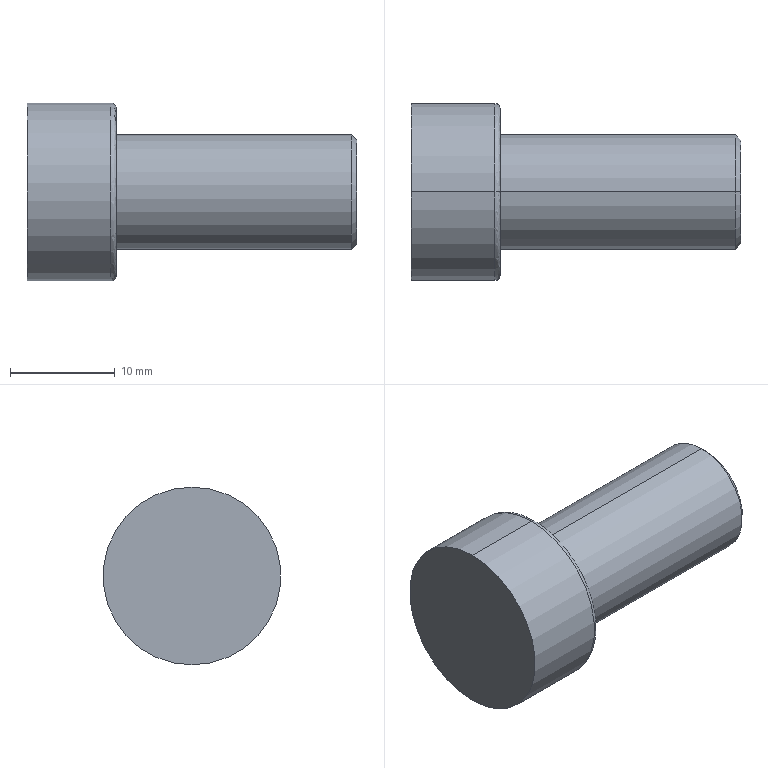Part | STEP file | _BMH070 Welle20 | 1 solid | 22 faces | box 31.5 x 17 x 17 mm | volume 3904 mm3 | cylinder 8 | cone 8 | plane 4 | spline 2 | commonest cylinder face diameters 3.242 x2 5.3 x2 11 x2 17 x2
STEP:
#1=CARTESIAN_POINT('',(8.5,0.,-8.));
#2=VERTEX_POINT('',#1);
#3=CARTESIAN_POINT('',(8.5,0.,8.));
#4=VERTEX_POINT('',#3);
#5=CARTESIAN_POINT('',(8.5,0.,-8.));
#6=CARTESIAN_POINT('',(8.5,-16.,-8.));
#7=CARTESIAN_POINT('',(8.5,-16.,8.));
#8=CARTESIAN_POINT('',(8.5,0.,8.));
#9=(BOUNDED_CURVE()B_SPLINE_CURVE(3,(#5,#6,#7,#8),.UNSPECIFIED.,.F.,.F.)B_SPLINE_CURVE_WITH_KNOTS((4,4),(0.,0.5),.UNSPECIFIED.)CURVE()GEOMETRIC_REPRESENTATION_ITEM()RATIONAL_B_SPLINE_CURVE((1.,0.3333,0.3333,1.))REPRESENTATION_ITEM(''));
#10=EDGE_CURVE('',#2,#4,#9,.T.);
#11=ORIENTED_EDGE('',*,*,#10,.T.);
#12=CARTESIAN_POINT('',(8.,0.,8.5));
#13=VERTEX_POINT('',#12);
#14=CARTESIAN_POINT('',(8.,0.,8.));
#15=DIRECTION('',(0.,-1.,0.));
#16=DIRECTION('',(0.,0.,1.));
#17=AXIS2_PLACEMENT_3D('',#14,#15,#16);
#18=CIRCLE('',#17,0.5);
#19=EDGE_CURVE('',#4,#13,#18,.T.);
#20=ORIENTED_EDGE('',*,*,#19,.T.);
#21=CARTESIAN_POINT('',(8.,0.,-8.5));
#22=VERTEX_POINT('',#21);
#23=CARTESIAN_POINT('',(8.,0.,0.));
#24=DIRECTION('',(1.,0.,0.));
#25=DIRECTION('',(0.,0.,-1.));
#26=AXIS2_PLACEMENT_3D('',#23,#24,#25);
#27=CIRCLE('',#26,8.5);
#28=EDGE_CURVE('',#13,#22,#27,.T.);
#29=ORIENTED_EDGE('',*,*,#28,.T.);
#30=CARTESIAN_POINT('',(8.,0.,-8.));
#31=DIRECTION('',(0.,1.,0.));
#32=DIRECTION('',(0.,0.,-1.));
#33=AXIS2_PLACEMENT_3D('',#30,#31,#32);
#34=CIRCLE('',#33,0.5);
#35=EDGE_CURVE('',#2,#22,#34,.T.);
#36=ORIENTED_EDGE('',*,*,#35,.F.);
#37=EDGE_LOOP('',(#11,#20,#29,#36));
#38=FACE_OUTER_BOUND('',#37,.T.);
#39=CARTESIAN_POINT('',(8.5,0.,8.));
#40=CARTESIAN_POINT('',(8.5,-16.,8.));
#41=CARTESIAN_POINT('',(8.5,-16.,-8.));
#42=CARTESIAN_POINT('',(8.5,0.,-8.));
#43=CARTESIAN_POINT('',(8.5,0.,8.293));
#44=CARTESIAN_POINT('',(8.5,-16.586,8.293));
#45=CARTESIAN_POINT('',(8.5,-16.586,-8.293));
#46=CARTESIAN_POINT('',(8.5,0.,-8.293));
#47=CARTESIAN_POINT('',(8.293,0.,8.5));
#48=CARTESIAN_POINT('',(8.293,-17.,8.5));
#49=CARTESIAN_POINT('',(8.293,-17.,-8.5));
#50=CARTESIAN_POINT('',(8.293,0.,-8.5));
#51=CARTESIAN_POINT('',(8.,0.,8.5));
#52=CARTESIAN_POINT('',(8.,-17.,8.5));
#53=CARTESIAN_POINT('',(8.,-17.,-8.5));
#54=CARTESIAN_POINT('',(8.,0.,-8.5));
#55=(BOUNDED_SURFACE()B_SPLINE_SURFACE(3,3,((#39,#40,#41,#42),(#43,#44,#45,#46),(#47,#48,#49,#50),(#51,#52,#53,#54)),.UNSPECIFIED.,.F.,.F.,.F.)B_SPLINE_SURFACE_WITH_KNOTS((4,4),(4,4),(0.,1.),(0.,1.),.UNSPECIFIED.)GEOMETRIC_REPRESENTATION_ITEM()RATIONAL_B_SPLINE_SURFACE(((1.,0.3333,0.3333,1.),(0.8047,0.2682,0.2682,0.8047),(0.8047,0.2682,0.2682,0.8047),(1.,0.3333,0.3333,1.)))REPRESENTATION_ITEM('')SURFACE());
#56=ADVANCED_FACE('',(#38),#55,.T.);
#57=CARTESIAN_POINT('',(31.,0.,5.5));
#58=VERTEX_POINT('',#57);
#59=CARTESIAN_POINT('',(31.,0.,-5.5));
#60=VERTEX_POINT('',#59);
#61=CARTESIAN_POINT('',(31.,0.,0.));
#62=DIRECTION('',(-1.,0.,0.));
#63=DIRECTION('',(0.,0.,1.));
#64=AXIS2_PLACEMENT_3D('',#61,#62,#63);
#65=CIRCLE('',#64,5.5);
#66=EDGE_CURVE('',#58,#60,#65,.T.);
#67=ORIENTED_EDGE('',*,*,#66,.T.);
#68=CARTESIAN_POINT('',(8.5,0.,-5.5));
#69=VERTEX_POINT('',#68);
#70=CARTESIAN_POINT('',(31.5,0.,-5.5));
#71=DIRECTION('',(-1.,0.,0.));
#72=VECTOR('',#71,1000.);
#73=LINE('',#70,#72);
#74=EDGE_CURVE('',#60,#69,#73,.T.);
#75=ORIENTED_EDGE('',*,*,#74,.T.);
#76=CARTESIAN_POINT('',(8.5,0.,5.5));
#77=VERTEX_POINT('',#76);
#78=CARTESIAN_POINT('',(8.5,0.,0.));
#79=DIRECTION('',(1.,0.,0.));
#80=DIRECTION('',(0.,0.,1.));
#81=AXIS2_PLACEMENT_3D('',#78,#79,#80);
#82=CIRCLE('',#81,5.5);
#83=EDGE_CURVE('',#69,#77,#82,.T.);
#84=ORIENTED_EDGE('',*,*,#83,.T.);
#85=CARTESIAN_POINT('',(31.5,0.,5.5));
#86=DIRECTION('',(-1.,0.,0.));
#87=VECTOR('',#86,1000.);
#88=LINE('',#85,#87);
#89=EDGE_CURVE('',#58,#77,#88,.T.);
#90=ORIENTED_EDGE('',*,*,#89,.F.);
#91=EDGE_LOOP('',(#67,#75,#84,#90));
#92=FACE_OUTER_BOUND('',#91,.T.);
#93=CARTESIAN_POINT('',(31.5,0.,0.));
#94=DIRECTION('',(-1.,0.,0.));
#95=DIRECTION('',(0.,0.,1.));
#96=AXIS2_PLACEMENT_3D('',#93,#94,#95);
#97=CYLINDRICAL_SURFACE('',#96,5.5);
#98=ADVANCED_FACE('',(#92),#97,.T.);
#99=CARTESIAN_POINT('',(31.5,0.,5.));
#100=VERTEX_POINT('',#99);
#101=CARTESIAN_POINT('',(31.5,0.,-5.));
#102=VERTEX_POINT('',#101);
#103=CARTESIAN_POINT('',(31.5,0.,0.));
#104=DIRECTION('',(-1.,0.,0.));
#105=DIRECTION('',(0.,0.,1.));
#106=AXIS2_PLACEMENT_3D('',#103,#104,#105);
#107=CIRCLE('',#106,5.);
#108=EDGE_CURVE('',#100,#102,#107,.T.);
#109=ORIENTED_EDGE('',*,*,#108,.T.);
#110=CARTESIAN_POINT('',(31.,0.,-5.5));
#111=DIRECTION('',(-0.7071,0.,-0.7071));
#112=VECTOR('',#111,1000.);
#113=LINE('',#110,#112);
#114=EDGE_CURVE('',#102,#60,#113,.T.);
#115=ORIENTED_EDGE('',*,*,#114,.T.);
#116=ORIENTED_EDGE('',*,*,#66,.F.);
#117=CARTESIAN_POINT('',(31.,0.,5.5));
#118=DIRECTION('',(-0.7071,0.,0.7071));
#119=VECTOR('',#118,1000.);
#120=LINE('',#117,#119);
#121=EDGE_CURVE('',#100,#58,#120,.T.);
#122=ORIENTED_EDGE('',*,*,#121,.F.);
#123=EDGE_LOOP('',(#109,#115,#116,#122));
#124=FACE_OUTER_BOUND('',#123,.T.);
#125=CARTESIAN_POINT('',(31.,0.,0.));
#126=DIRECTION('',(-1.,0.,0.));
#127=DIRECTION('',(0.,0.,1.));
#128=AXIS2_PLACEMENT_3D('',#125,#126,#127);
#129=CONICAL_SURFACE('',#128,5.5,0.7854);
#130=ADVANCED_FACE('',(#124),#129,.T.);
#131=CARTESIAN_POINT('',(8.,0.,0.));
#132=DIRECTION('',(1.,0.,0.));
#133=DIRECTION('',(0.,0.,-1.));
#134=AXIS2_PLACEMENT_3D('',#131,#132,#133);
#135=CIRCLE('',#134,8.5);
#136=EDGE_CURVE('',#22,#13,#135,.T.);
#137=ORIENTED_EDGE('',*,*,#136,.F.);
#138=CARTESIAN_POINT('',(0.,0.,-8.5));
#139=VERTEX_POINT('',#138);
#140=CARTESIAN_POINT('',(31.5,0.,-8.5));
#141=DIRECTION('',(-1.,0.,0.));
#142=VECTOR('',#141,1000.);
#143=LINE('',#140,#142);
#144=EDGE_CURVE('',#22,#139,#143,.T.);
#145=ORIENTED_EDGE('',*,*,#144,.T.);
#146=CARTESIAN_POINT('',(0.,0.,8.5));
#147=VERTEX_POINT('',#146);
#148=CARTESIAN_POINT('',(0.,0.,0.));
#149=DIRECTION('',(1.,0.,0.));
#150=DIRECTION('',(0.,0.,1.));
#151=AXIS2_PLACEMENT_3D('',#148,#149,#150);
#152=CIRCLE('',#151,8.5);
#153=EDGE_CURVE('',#139,#147,#152,.T.);
#154=ORIENTED_EDGE('',*,*,#153,.T.);
#155=CARTESIAN_POINT('',(31.5,0.,8.5));
#156=DIRECTION('',(-1.,0.,0.));
#157=VECTOR('',#156,1000.);
#158=LINE('',#155,#157);
#159=EDGE_CURVE('',#13,#147,#158,.T.);
#160=ORIENTED_EDGE('',*,*,#159,.F.);
#161=EDGE_LOOP('',(#137,#145,#154,#160));
#162=FACE_OUTER_BOUND('',#161,.T.);
#163=CARTESIAN_POINT('',(31.5,0.,0.));
#164=DIRECTION('',(-1.,0.,0.));
#165=DIRECTION('',(0.,0.,1.));
#166=AXIS2_PLACEMENT_3D('',#163,#164,#165);
#167=CYLINDRICAL_SURFACE('',#166,8.5);
#168=ADVANCED_FACE('',(#162),#167,.T.);
#169=CARTESIAN_POINT('',(29.4,0.,2.65));
#170=VERTEX_POINT('',#169);
#171=CARTESIAN_POINT('',(29.4,0.,-2.65));
#172=VERTEX_POINT('',#171);
#173=CARTESIAN_POINT('',(29.4,0.,0.));
#174=DIRECTION('',(1.,0.,0.));
#175=DIRECTION('',(0.,0.,-1.));
#176=AXIS2_PLACEMENT_3D('',#173,#174,#175);
#177=CIRCLE('',#176,2.65);
#178=EDGE_CURVE('',#170,#172,#177,.T.);
#179=ORIENTED_EDGE('',*,*,#178,.F.);
#180=CARTESIAN_POINT('',(31.5,0.,3.862));
#181=VERTEX_POINT('',#180);
#182=CARTESIAN_POINT('',(31.5,0.,3.862));
#183=DIRECTION('',(0.866,0.,0.5));
#184=VECTOR('',#183,1000.);
#185=LINE('',#182,#184);
#186=EDGE_CURVE('',#170,#181,#185,.T.);
#187=ORIENTED_EDGE('',*,*,#186,.T.);
#188=CARTESIAN_POINT('',(31.5,0.,-3.862));
#189=VERTEX_POINT('',#188);
#190=CARTESIAN_POINT('',(31.5,0.,0.));
#191=DIRECTION('',(1.,0.,0.));
#192=DIRECTION('',(0.,0.,-1.));
#193=AXIS2_PLACEMENT_3D('',#190,#191,#192);
#194=CIRCLE('',#193,3.862);
#195=EDGE_CURVE('',#181,#189,#194,.T.);
#196=ORIENTED_EDGE('',*,*,#195,.T.);
#197=CARTESIAN_POINT('',(31.5,0.,-3.862));
#198=DIRECTION('',(0.866,0.,-0.5));
#199=VECTOR('',#198,1000.);
#200=LINE('',#197,#199);
#201=EDGE_CURVE('',#172,#189,#200,.T.);
#202=ORIENTED_EDGE('',*,*,#201,.F.);
#203=EDGE_LOOP('',(#179,#187,#196,#202));
#204=FACE_OUTER_BOUND('',#203,.T.);
#205=CARTESIAN_POINT('',(31.5,0.,0.));
#206=DIRECTION('',(1.,0.,0.));
#207=DIRECTION('',(0.,0.,-1.));
#208=AXIS2_PLACEMENT_3D('',#205,#206,#207);
#209=CONICAL_SURFACE('',#208,3.862,0.5236);
#210=ADVANCED_FACE('',(#204),#209,.F.);
#211=ORIENTED_EDGE('',*,*,#178,.T.);
#212=CARTESIAN_POINT('',(27.8,0.,-2.65));
#213=VERTEX_POINT('',#212);
#214=CARTESIAN_POINT('',(31.5,0.,-2.65));
#215=DIRECTION('',(-1.,0.,0.));
#216=VECTOR('',#215,1000.);
#217=LINE('',#214,#216);
#218=EDGE_CURVE('',#172,#213,#217,.T.);
#219=ORIENTED_EDGE('',*,*,#218,.T.);
#220=CARTESIAN_POINT('',(27.8,0.,2.65));
#221=VERTEX_POINT('',#220);
#222=CARTESIAN_POINT('',(27.8,0.,0.));
#223=DIRECTION('',(1.,0.,0.));
#224=DIRECTION('',(0.,0.,1.));
#225=AXIS2_PLACEMENT_3D('',#222,#223,#224);
#226=CIRCLE('',#225,2.65);
#227=EDGE_CURVE('',#221,#213,#226,.T.);
#228=ORIENTED_EDGE('',*,*,#227,.F.);
#229=CARTESIAN_POINT('',(31.5,0.,2.65));
#230=DIRECTION('',(-1.,0.,0.));
#231=VECTOR('',#230,1000.);
#232=LINE('',#229,#231);
#233=EDGE_CURVE('',#170,#221,#232,.T.);
#234=ORIENTED_EDGE('',*,*,#233,.F.);
#235=EDGE_LOOP('',(#211,#219,#228,#234));
#236=FACE_OUTER_BOUND('',#235,.T.);
#237=CARTESIAN_POINT('',(31.5,0.,0.));
#238=DIRECTION('',(-1.,0.,0.));
#239=DIRECTION('',(0.,0.,1.));
#240=AXIS2_PLACEMENT_3D('',#237,#238,#239);
#241=CYLINDRICAL_SURFACE('',#240,2.65);
#242=ADVANCED_FACE('',(#236),#241,.F.);
#243=CARTESIAN_POINT('',(27.421,0.,1.621));
#244=VERTEX_POINT('',#243);
#245=CARTESIAN_POINT('',(27.421,0.,-1.621));
#246=VERTEX_POINT('',#245);
#247=CARTESIAN_POINT('',(27.421,0.,0.));
#248=DIRECTION('',(1.,0.,0.));
#249=DIRECTION('',(0.,0.,-1.));
#250=AXIS2_PLACEMENT_3D('',#247,#248,#249);
#251=CIRCLE('',#250,1.621);
#252=EDGE_CURVE('',#244,#246,#251,.T.);
#253=ORIENTED_EDGE('',*,*,#252,.F.);
#254=CARTESIAN_POINT('',(27.8,0.,2.));
#255=VERTEX_POINT('',#254);
#256=CARTESIAN_POINT('',(27.8,0.,2.));
#257=DIRECTION('',(0.7071,0.,0.7071));
#258=VECTOR('',#257,1000.);
#259=LINE('',#256,#258);
#260=EDGE_CURVE('',#244,#255,#259,.T.);
#261=ORIENTED_EDGE('',*,*,#260,.T.);
#262=CARTESIAN_POINT('',(27.8,0.,-2.));
#263=VERTEX_POINT('',#262);
#264=CARTESIAN_POINT('',(27.8,0.,0.));
#265=DIRECTION('',(-1.,0.,0.));
#266=DIRECTION('',(0.,0.,-1.));
#267=AXIS2_PLACEMENT_3D('',#264,#265,#266);
#268=CIRCLE('',#267,2.);
#269=EDGE_CURVE('',#263,#255,#268,.T.);
#270=ORIENTED_EDGE('',*,*,#269,.F.);
#271=CARTESIAN_POINT('',(27.8,0.,-2.));
#272=DIRECTION('',(0.7071,0.,-0.7071));
#273=VECTOR('',#272,1000.);
#274=LINE('',#271,#273);
#275=EDGE_CURVE('',#246,#263,#274,.T.);
#276=ORIENTED_EDGE('',*,*,#275,.F.);
#277=EDGE_LOOP('',(#253,#261,#270,#276));
#278=FACE_OUTER_BOUND('',#277,.T.);
#279=CARTESIAN_POINT('',(27.8,0.,0.));
#280=DIRECTION('',(1.,0.,0.));
#281=DIRECTION('',(0.,0.,-1.));
#282=AXIS2_PLACEMENT_3D('',#279,#280,#281);
#283=CONICAL_SURFACE('',#282,2.,0.7854);
#284=ADVANCED_FACE('',(#278),#283,.F.);
#285=ORIENTED_EDGE('',*,*,#252,.T.);
#286=CARTESIAN_POINT('',(16.3,0.,-1.621));
#287=VERTEX_POINT('',#286);
#288=CARTESIAN_POINT('',(31.5,0.,-1.621));
#289=DIRECTION('',(-1.,0.,0.));
#290=VECTOR('',#289,1000.);
#291=LINE('',#288,#290);
#292=EDGE_CURVE('',#246,#287,#291,.T.);
#293=ORIENTED_EDGE('',*,*,#292,.T.);
#294=CARTESIAN_POINT('',(16.3,0.,1.621));
#295=VERTEX_POINT('',#294);
#296=CARTESIAN_POINT('',(16.3,0.,0.));
#297=DIRECTION('',(1.,0.,0.));
#298=DIRECTION('',(0.,0.,1.));
#299=AXIS2_PLACEMENT_3D('',#296,#297,#298);
#300=CIRCLE('',#299,1.621);
#301=EDGE_CURVE('',#295,#287,#300,.T.);
#302=ORIENTED_EDGE('',*,*,#301,.F.);
#303=CARTESIAN_POINT('',(31.5,0.,1.621));
#304=DIRECTION('',(-1.,0.,0.));
#305=VECTOR('',#304,1000.);
#306=LINE('',#303,#305);
#307=EDGE_CURVE('',#244,#295,#306,.T.);
#308=ORIENTED_EDGE('',*,*,#307,.F.);
#309=EDGE_LOOP('',(#285,#293,#302,#308));
#310=FACE_OUTER_BOUND('',#309,.T.);
#311=CARTESIAN_POINT('',(31.5,0.,0.));
#312=DIRECTION('',(-1.,0.,0.));
#313=DIRECTION('',(0.,0.,1.));
#314=AXIS2_PLACEMENT_3D('',#311,#312,#313);
#315=CYLINDRICAL_SURFACE('',#314,1.621);
#316=ADVANCED_FACE('',(#310),#315,.F.);
#317=CARTESIAN_POINT('',(15.364,0.,0.));
#318=VERTEX_POINT('',#317);
#319=CARTESIAN_POINT('',(16.3,0.,-1.621));
#320=DIRECTION('',(0.5,0.,-0.866));
#321=VECTOR('',#320,1000.);
#322=LINE('',#319,#321);
#323=EDGE_CURVE('',#318,#287,#322,.T.);
#324=ORIENTED_EDGE('',*,*,#323,.F.);
#325=CARTESIAN_POINT('',(16.3,0.,1.621));
#326=DIRECTION('',(0.5,0.,0.866));
#327=VECTOR('',#326,1000.);
#328=LINE('',#325,#327);
#329=EDGE_CURVE('',#318,#295,#328,.T.);
#330=ORIENTED_EDGE('',*,*,#329,.T.);
#331=ORIENTED_EDGE('',*,*,#301,.T.);
#332=EDGE_LOOP('',(#324,#330,#331));
#333=FACE_OUTER_BOUND('',#332,.T.);
#334=CARTESIAN_POINT('',(16.3,0.,0.));
#335=DIRECTION('',(1.,0.,0.));
#336=DIRECTION('',(0.,0.,-1.));
#337=AXIS2_PLACEMENT_3D('',#334,#335,#336);
#338=CONICAL_SURFACE('',#337,1.621,1.047);
#339=ADVANCED_FACE('',(#333),#338,.F.);
#340=ORIENTED_EDGE('',*,*,#74,.F.);
#341=CARTESIAN_POINT('',(31.,0.,0.));
#342=DIRECTION('',(-1.,0.,0.));
#343=DIRECTION('',(0.,0.,1.));
#344=AXIS2_PLACEMENT_3D('',#341,#342,#343);
#345=CIRCLE('',#344,5.5);
#346=EDGE_CURVE('',#60,#58,#345,.T.);
#347=ORIENTED_EDGE('',*,*,#346,.T.);
#348=ORIENTED_EDGE('',*,*,#89,.T.);
#349=CARTESIAN_POINT('',(8.5,0.,0.));
#350=DIRECTION('',(1.,0.,0.));
#351=DIRECTION('',(0.,0.,1.));
#352=AXIS2_PLACEMENT_3D('',#349,#350,#351);
#353=CIRCLE('',#352,5.5);
#354=EDGE_CURVE('',#77,#69,#353,.T.);
#355=ORIENTED_EDGE('',*,*,#354,.T.);
#356=EDGE_LOOP('',(#340,#347,#348,#355));
#357=FACE_OUTER_BOUND('',#356,.T.);
#358=CARTESIAN_POINT('',(31.5,0.,0.));
#359=DIRECTION('',(-1.,0.,0.));
#360=DIRECTION('',(0.,0.,1.));
#361=AXIS2_PLACEMENT_3D('',#358,#359,#360);
#362=CYLINDRICAL_SURFACE('',#361,5.5);
#363=ADVANCED_FACE('',(#357),#362,.T.);
#364=ORIENTED_EDGE('',*,*,#10,.F.);
#365=CARTESIAN_POINT('',(8.5,0.,8.));
#366=CARTESIAN_POINT('',(8.5,16.,8.));
#367=CARTESIAN_POINT('',(8.5,16.,-8.));
#368=CARTESIAN_POINT('',(8.5,0.,-8.));
#369=(BOUNDED_CURVE()B_SPLINE_CURVE(3,(#365,#366,#367,#368),.UNSPECIFIED.,.F.,.F.)B_SPLINE_CURVE_WITH_KNOTS((4,4),(0.5,1.),.UNSPECIFIED.)CURVE()GEOMETRIC_REPRESENTATION_ITEM()RATIONAL_B_SPLINE_CURVE((1.,0.3333,0.3333,1.))REPRESENTATION_ITEM(''));
#370=EDGE_CURVE('',#4,#2,#369,.T.);
#371=ORIENTED_EDGE('',*,*,#370,.F.);
#372=EDGE_LOOP('',(#364,#371));
#373=FACE_OUTER_BOUND('',#372,.T.);
#374=ORIENTED_EDGE('',*,*,#354,.F.);
#375=ORIENTED_EDGE('',*,*,#83,.F.);
#376=EDGE_LOOP('',(#374,#375));
#377=FACE_BOUND('',#376,.T.);
#378=CARTESIAN_POINT('',(8.5,8.,0.));
#379=DIRECTION('',(-1.,0.,0.));
#380=DIRECTION('',(0.,0.,1.));
#381=AXIS2_PLACEMENT_3D('',#378,#379,#380);
#382=PLANE('',#381);
#383=ADVANCED_FACE('',(#373,#377),#382,.F.);
#384=ORIENTED_EDGE('',*,*,#114,.F.);
#385=CARTESIAN_POINT('',(31.5,0.,0.));
#386=DIRECTION('',(-1.,0.,0.));
#387=DIRECTION('',(0.,0.,1.));
#388=AXIS2_PLACEMENT_3D('',#385,#386,#387);
#389=CIRCLE('',#388,5.);
#390=EDGE_CURVE('',#102,#100,#389,.T.);
#391=ORIENTED_EDGE('',*,*,#390,.T.);
#392=ORIENTED_EDGE('',*,*,#121,.T.);
#393=ORIENTED_EDGE('',*,*,#346,.F.);
#394=EDGE_LOOP('',(#384,#391,#392,#393));
#395=FACE_OUTER_BOUND('',#394,.T.);
#396=CARTESIAN_POINT('',(31.,0.,0.));
#397=DIRECTION('',(-1.,0.,0.));
#398=DIRECTION('',(0.,0.,1.));
#399=AXIS2_PLACEMENT_3D('',#396,#397,#398);
#400=CONICAL_SURFACE('',#399,5.5,0.7854);
#401=ADVANCED_FACE('',(#395),#400,.T.);
#402=ORIENTED_EDGE('',*,*,#19,.F.);
#403=ORIENTED_EDGE('',*,*,#370,.T.);
#404=ORIENTED_EDGE('',*,*,#35,.T.);
#405=ORIENTED_EDGE('',*,*,#136,.T.);
#406=EDGE_LOOP('',(#402,#403,#404,#405));
#407=FACE_OUTER_BOUND('',#406,.T.);
#408=CARTESIAN_POINT('',(8.5,0.,-8.));
#409=CARTESIAN_POINT('',(8.5,16.,-8.));
#410=CARTESIAN_POINT('',(8.5,16.,8.));
#411=CARTESIAN_POINT('',(8.5,0.,8.));
#412=CARTESIAN_POINT('',(8.5,0.,-8.293));
#413=CARTESIAN_POINT('',(8.5,16.586,-8.293));
#414=CARTESIAN_POINT('',(8.5,16.586,8.293));
#415=CARTESIAN_POINT('',(8.5,0.,8.293));
#416=CARTESIAN_POINT('',(8.293,0.,-8.5));
#417=CARTESIAN_POINT('',(8.293,17.,-8.5));
#418=CARTESIAN_POINT('',(8.293,17.,8.5));
#419=CARTESIAN_POINT('',(8.293,0.,8.5));
#420=CARTESIAN_POINT('',(8.,0.,-8.5));
#421=CARTESIAN_POINT('',(8.,17.,-8.5));
#422=CARTESIAN_POINT('',(8.,17.,8.5));
#423=CARTESIAN_POINT('',(8.,0.,8.5));
#424=(BOUNDED_SURFACE()B_SPLINE_SURFACE(3,3,((#408,#409,#410,#411),(#412,#413,#414,#415),(#416,#417,#418,#419),(#420,#421,#422,#423)),.UNSPECIFIED.,.F.,.F.,.F.)B_SPLINE_SURFACE_WITH_KNOTS((4,4),(4,4),(0.,1.),(0.,1.),.UNSPECIFIED.)GEOMETRIC_REPRESENTATION_ITEM()RATIONAL_B_SPLINE_SURFACE(((1.,0.3333,0.3333,1.),(0.8047,0.2682,0.2682,0.8047),(0.8047,0.2682,0.2682,0.8047),(1.,0.3333,0.3333,1.)))REPRESENTATION_ITEM('')SURFACE());
#425=ADVANCED_FACE('',(#407),#424,.T.);
#426=ORIENTED_EDGE('',*,*,#108,.F.);
#427=ORIENTED_EDGE('',*,*,#390,.F.);
#428=EDGE_LOOP('',(#426,#427));
#429=FACE_OUTER_BOUND('',#428,.T.);
#430=CARTESIAN_POINT('',(31.5,0.,0.));
#431=DIRECTION('',(1.,0.,0.));
#432=DIRECTION('',(0.,0.,-1.));
#433=AXIS2_PLACEMENT_3D('',#430,#431,#432);
#434=CIRCLE('',#433,3.862);
#435=EDGE_CURVE('',#189,#181,#434,.T.);
#436=ORIENTED_EDGE('',*,*,#435,.F.);
#437=ORIENTED_EDGE('',*,*,#195,.F.);
#438=EDGE_LOOP('',(#436,#437));
#439=FACE_BOUND('',#438,.T.);
#440=CARTESIAN_POINT('',(31.5,5.,0.));
#441=DIRECTION('',(-1.,0.,0.));
#442=DIRECTION('',(0.,0.,1.));
#443=AXIS2_PLACEMENT_3D('',#440,#441,#442);
#444=PLANE('',#443);
#445=ADVANCED_FACE('',(#429,#439),#444,.F.);
#446=ORIENTED_EDGE('',*,*,#144,.F.);
#447=ORIENTED_EDGE('',*,*,#28,.F.);
#448=ORIENTED_EDGE('',*,*,#159,.T.);
#449=CARTESIAN_POINT('',(0.,0.,0.));
#450=DIRECTION('',(1.,0.,0.));
#451=DIRECTION('',(0.,0.,1.));
#452=AXIS2_PLACEMENT_3D('',#449,#450,#451);
#453=CIRCLE('',#452,8.5);
#454=EDGE_CURVE('',#147,#139,#453,.T.);
#455=ORIENTED_EDGE('',*,*,#454,.T.);
#456=EDGE_LOOP('',(#446,#447,#448,#455));
#457=FACE_OUTER_BOUND('',#456,.T.);
#458=CARTESIAN_POINT('',(31.5,0.,0.));
#459=DIRECTION('',(-1.,0.,0.));
#460=DIRECTION('',(0.,0.,1.));
#461=AXIS2_PLACEMENT_3D('',#458,#459,#460);
#462=CYLINDRICAL_SURFACE('',#461,8.5);
#463=ADVANCED_FACE('',(#457),#462,.T.);
#464=ORIENTED_EDGE('',*,*,#186,.F.);
#465=CARTESIAN_POINT('',(29.4,0.,0.));
#466=DIRECTION('',(1.,0.,0.));
#467=DIRECTION('',(0.,0.,-1.));
#468=AXIS2_PLACEMENT_3D('',#465,#466,#467);
#469=CIRCLE('',#468,2.65);
#470=EDGE_CURVE('',#172,#170,#469,.T.);
#471=ORIENTED_EDGE('',*,*,#470,.F.);
#472=ORIENTED_EDGE('',*,*,#201,.T.);
#473=ORIENTED_EDGE('',*,*,#435,.T.);
#474=EDGE_LOOP('',(#464,#471,#472,#473));
#475=FACE_OUTER_BOUND('',#474,.T.);
#476=CARTESIAN_POINT('',(31.5,0.,0.));
#477=DIRECTION('',(1.,0.,0.));
#478=DIRECTION('',(0.,0.,-1.));
#479=AXIS2_PLACEMENT_3D('',#476,#477,#478);
#480=CONICAL_SURFACE('',#479,3.862,0.5236);
#481=ADVANCED_FACE('',(#475),#480,.F.);
#482=ORIENTED_EDGE('',*,*,#454,.F.);
#483=ORIENTED_EDGE('',*,*,#153,.F.);
#484=EDGE_LOOP('',(#482,#483));
#485=FACE_OUTER_BOUND('',#484,.T.);
#486=CARTESIAN_POINT('',(0.,0.,0.));
#487=DIRECTION('',(1.,0.,0.));
#488=DIRECTION('',(0.,0.,-1.));
#489=AXIS2_PLACEMENT_3D('',#486,#487,#488);
#490=PLANE('',#489);
#491=ADVANCED_FACE('',(#485),#490,.F.);
#492=ORIENTED_EDGE('',*,*,#218,.F.);
#493=ORIENTED_EDGE('',*,*,#470,.T.);
#494=ORIENTED_EDGE('',*,*,#233,.T.);
#495=CARTESIAN_POINT('',(27.8,0.,0.));
#496=DIRECTION('',(1.,0.,0.));
#497=DIRECTION('',(0.,0.,1.));
#498=AXIS2_PLACEMENT_3D('',#495,#496,#497);
#499=CIRCLE('',#498,2.65);
#500=EDGE_CURVE('',#213,#221,#499,.T.);
#501=ORIENTED_EDGE('',*,*,#500,.F.);
#502=EDGE_LOOP('',(#492,#493,#494,#501));
#503=FACE_OUTER_BOUND('',#502,.T.);
#504=CARTESIAN_POINT('',(31.5,0.,0.));
#505=DIRECTION('',(-1.,0.,0.));
#506=DIRECTION('',(0.,0.,1.));
#507=AXIS2_PLACEMENT_3D('',#504,#505,#506);
#508=CYLINDRICAL_SURFACE('',#507,2.65);
#509=ADVANCED_FACE('',(#503),#508,.F.);
#510=ORIENTED_EDGE('',*,*,#269,.T.);
#511=CARTESIAN_POINT('',(27.8,0.,0.));
#512=DIRECTION('',(-1.,0.,0.));
#513=DIRECTION('',(0.,0.,-1.));
#514=AXIS2_PLACEMENT_3D('',#511,#512,#513);
#515=CIRCLE('',#514,2.);
#516=EDGE_CURVE('',#255,#263,#515,.T.);
#517=ORIENTED_EDGE('',*,*,#516,.T.);
#518=EDGE_LOOP('',(#510,#517));
#519=FACE_BOUND('',#518,.T.);
#520=ORIENTED_EDGE('',*,*,#227,.T.);
#521=ORIENTED_EDGE('',*,*,#500,.T.);
#522=EDGE_LOOP('',(#520,#521));
#523=FACE_OUTER_BOUND('',#522,.T.);
#524=CARTESIAN_POINT('',(27.8,2.,0.));
#525=DIRECTION('',(1.,0.,0.));
#526=DIRECTION('',(0.,0.,-1.));
#527=AXIS2_PLACEMENT_3D('',#524,#525,#526);
#528=PLANE('',#527);
#529=ADVANCED_FACE('',(#519,#523),#528,.T.);
#530=ORIENTED_EDGE('',*,*,#260,.F.);
#531=CARTESIAN_POINT('',(27.421,0.,0.));
#532=DIRECTION('',(1.,0.,0.));
#533=DIRECTION('',(0.,0.,-1.));
#534=AXIS2_PLACEMENT_3D('',#531,#532,#533);
#535=CIRCLE('',#534,1.621);
#536=EDGE_CURVE('',#246,#244,#535,.T.);
#537=ORIENTED_EDGE('',*,*,#536,.F.);
#538=ORIENTED_EDGE('',*,*,#275,.T.);
#539=ORIENTED_EDGE('',*,*,#516,.F.);
#540=EDGE_LOOP('',(#530,#537,#538,#539));
#541=FACE_OUTER_BOUND('',#540,.T.);
#542=CARTESIAN_POINT('',(27.8,0.,0.));
#543=DIRECTION('',(1.,0.,0.));
#544=DIRECTION('',(0.,0.,-1.));
#545=AXIS2_PLACEMENT_3D('',#542,#543,#544);
#546=CONICAL_SURFACE('',#545,2.,0.7854);
#547=ADVANCED_FACE('',(#541),#546,.F.);
#548=ORIENTED_EDGE('',*,*,#292,.F.);
#549=ORIENTED_EDGE('',*,*,#536,.T.);
#550=ORIENTED_EDGE('',*,*,#307,.T.);
#551=CARTESIAN_POINT('',(16.3,0.,0.));
#552=DIRECTION('',(1.,0.,0.));
#553=DIRECTION('',(0.,0.,1.));
#554=AXIS2_PLACEMENT_3D('',#551,#552,#553);
#555=CIRCLE('',#554,1.621);
#556=EDGE_CURVE('',#287,#295,#555,.T.);
#557=ORIENTED_EDGE('',*,*,#556,.F.);
#558=EDGE_LOOP('',(#548,#549,#550,#557));
#559=FACE_OUTER_BOUND('',#558,.T.);
#560=CARTESIAN_POINT('',(31.5,0.,0.));
#561=DIRECTION('',(-1.,0.,0.));
#562=DIRECTION('',(0.,0.,1.));
#563=AXIS2_PLACEMENT_3D('',#560,#561,#562);
#564=CYLINDRICAL_SURFACE('',#563,1.621);
#565=ADVANCED_FACE('',(#559),#564,.F.);
#566=ORIENTED_EDGE('',*,*,#329,.F.);
#567=ORIENTED_EDGE('',*,*,#323,.T.);
#568=ORIENTED_EDGE('',*,*,#556,.T.);
#569=EDGE_LOOP('',(#566,#567,#568));
#570=FACE_OUTER_BOUND('',#569,.T.);
#571=CARTESIAN_POINT('',(16.3,0.,0.));
#572=DIRECTION('',(1.,0.,0.));
#573=DIRECTION('',(0.,0.,-1.));
#574=AXIS2_PLACEMENT_3D('',#571,#572,#573);
#575=CONICAL_SURFACE('',#574,1.621,1.047);
#576=ADVANCED_FACE('',(#570),#575,.F.);
#577=CLOSED_SHELL('',(#56,#98,#130,#168,#210,#242,#284,#316,#339,#363,#383,#401,#425,#445,#463,#481,#491,#509,#529,#547,#565,#576));
#578=MANIFOLD_SOLID_BREP('',#577);
#579=CARTESIAN_POINT('',(0.,0.,0.));
#580=DIRECTION('',(0.,0.,1.));
#581=DIRECTION('',(1.,0.,0.));
#582=AXIS2_PLACEMENT_3D('',#579,#580,#581);
#583=(LENGTH_UNIT()NAMED_UNIT(*)SI_UNIT(.MILLI.,.METRE.));
#584=UNCERTAINTY_MEASURE_WITH_UNIT(LENGTH_MEASURE(0.00001),#583,'','');
#585=(NAMED_UNIT(*)PLANE_ANGLE_UNIT()SI_UNIT($,.RADIAN.));
#586=(NAMED_UNIT(*)SI_UNIT($,.STERADIAN.)SOLID_ANGLE_UNIT());
#587=(GEOMETRIC_REPRESENTATION_CONTEXT(3)GLOBAL_UNCERTAINTY_ASSIGNED_CONTEXT((#584))GLOBAL_UNIT_ASSIGNED_CONTEXT((#583,#585,#586))REPRESENTATION_CONTEXT('',''));
#588=ADVANCED_BREP_SHAPE_REPRESENTATION('',(#578,#582),#587);